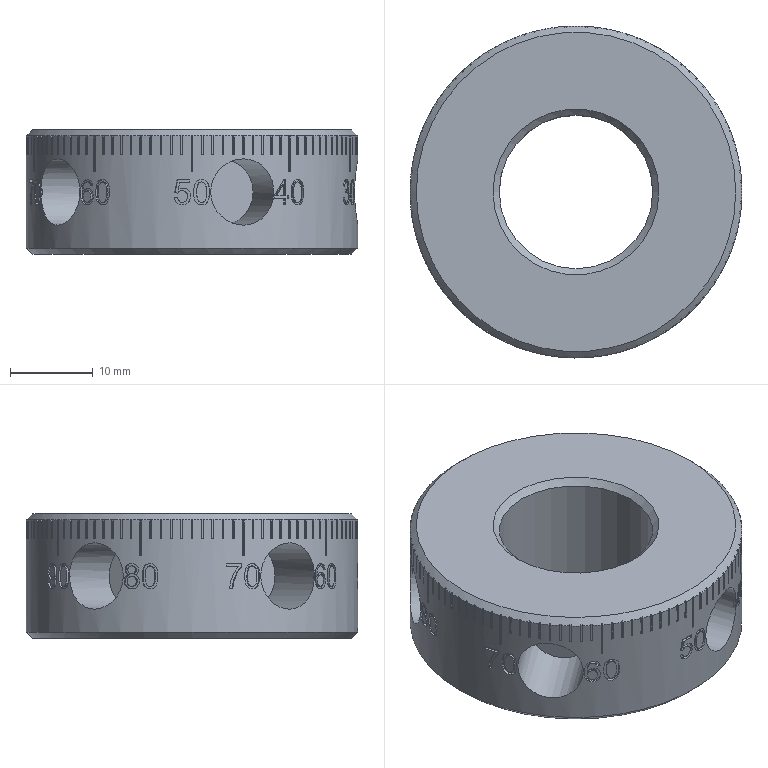Part | STEP file | 冲床-300配套压波_id638_x_t | 1 solid | 535 faces | box 40 x 40 x 15 mm | volume 12585 mm3 | plane 435 | spline 55 | cylinder 41 | cone 4 | commonest cylinder face diameters 39.4 x19 40 x16 8 x5 18.5 x1